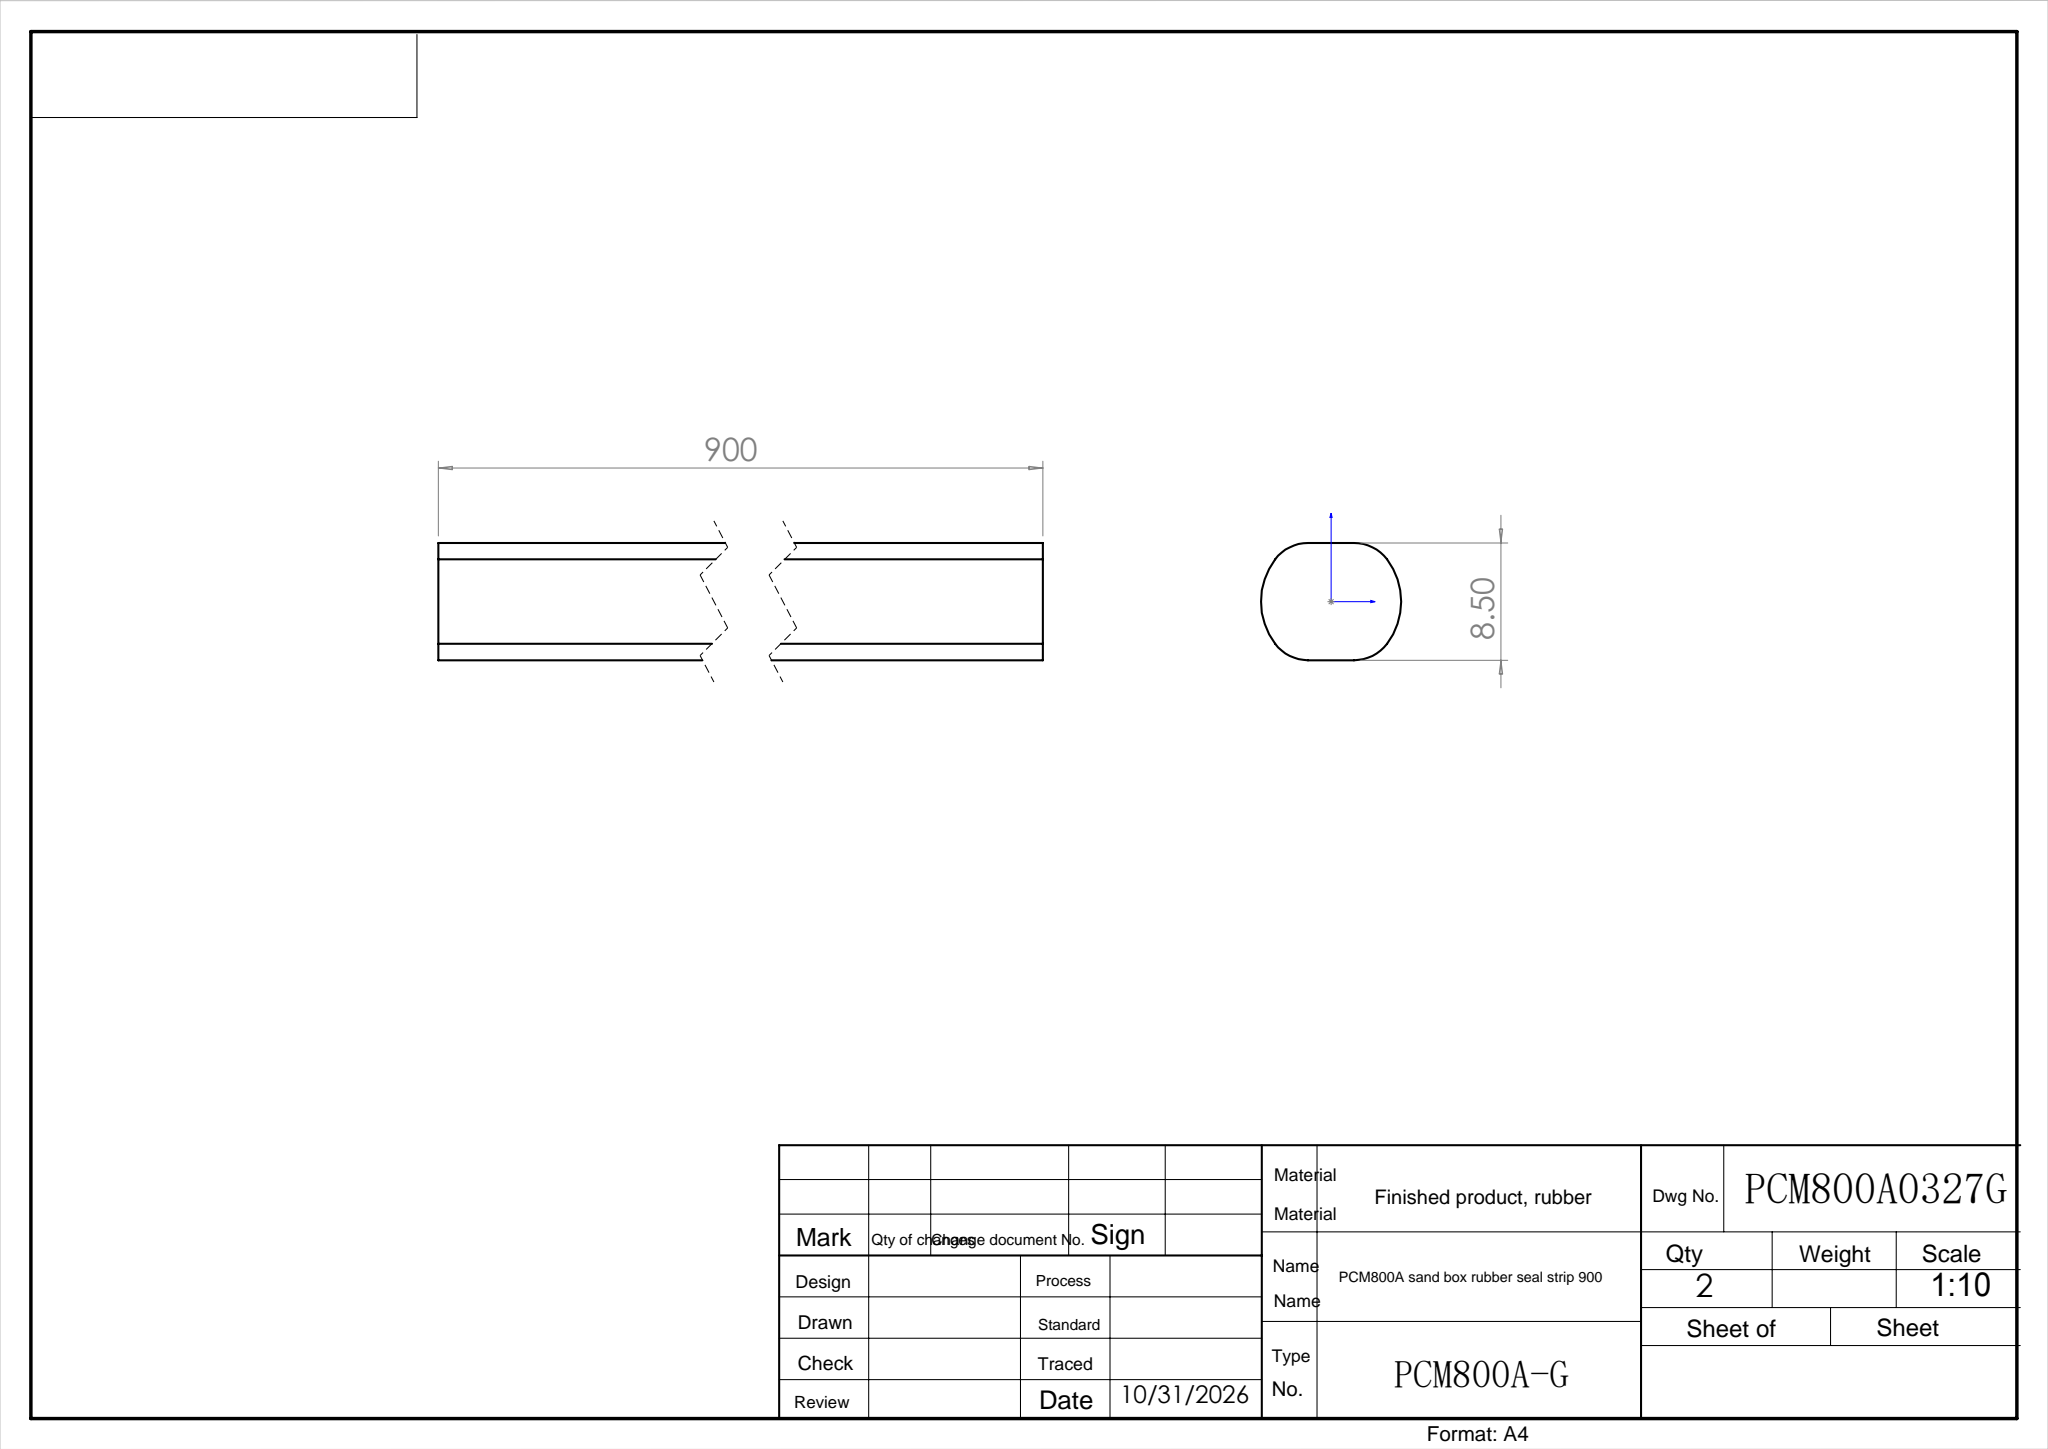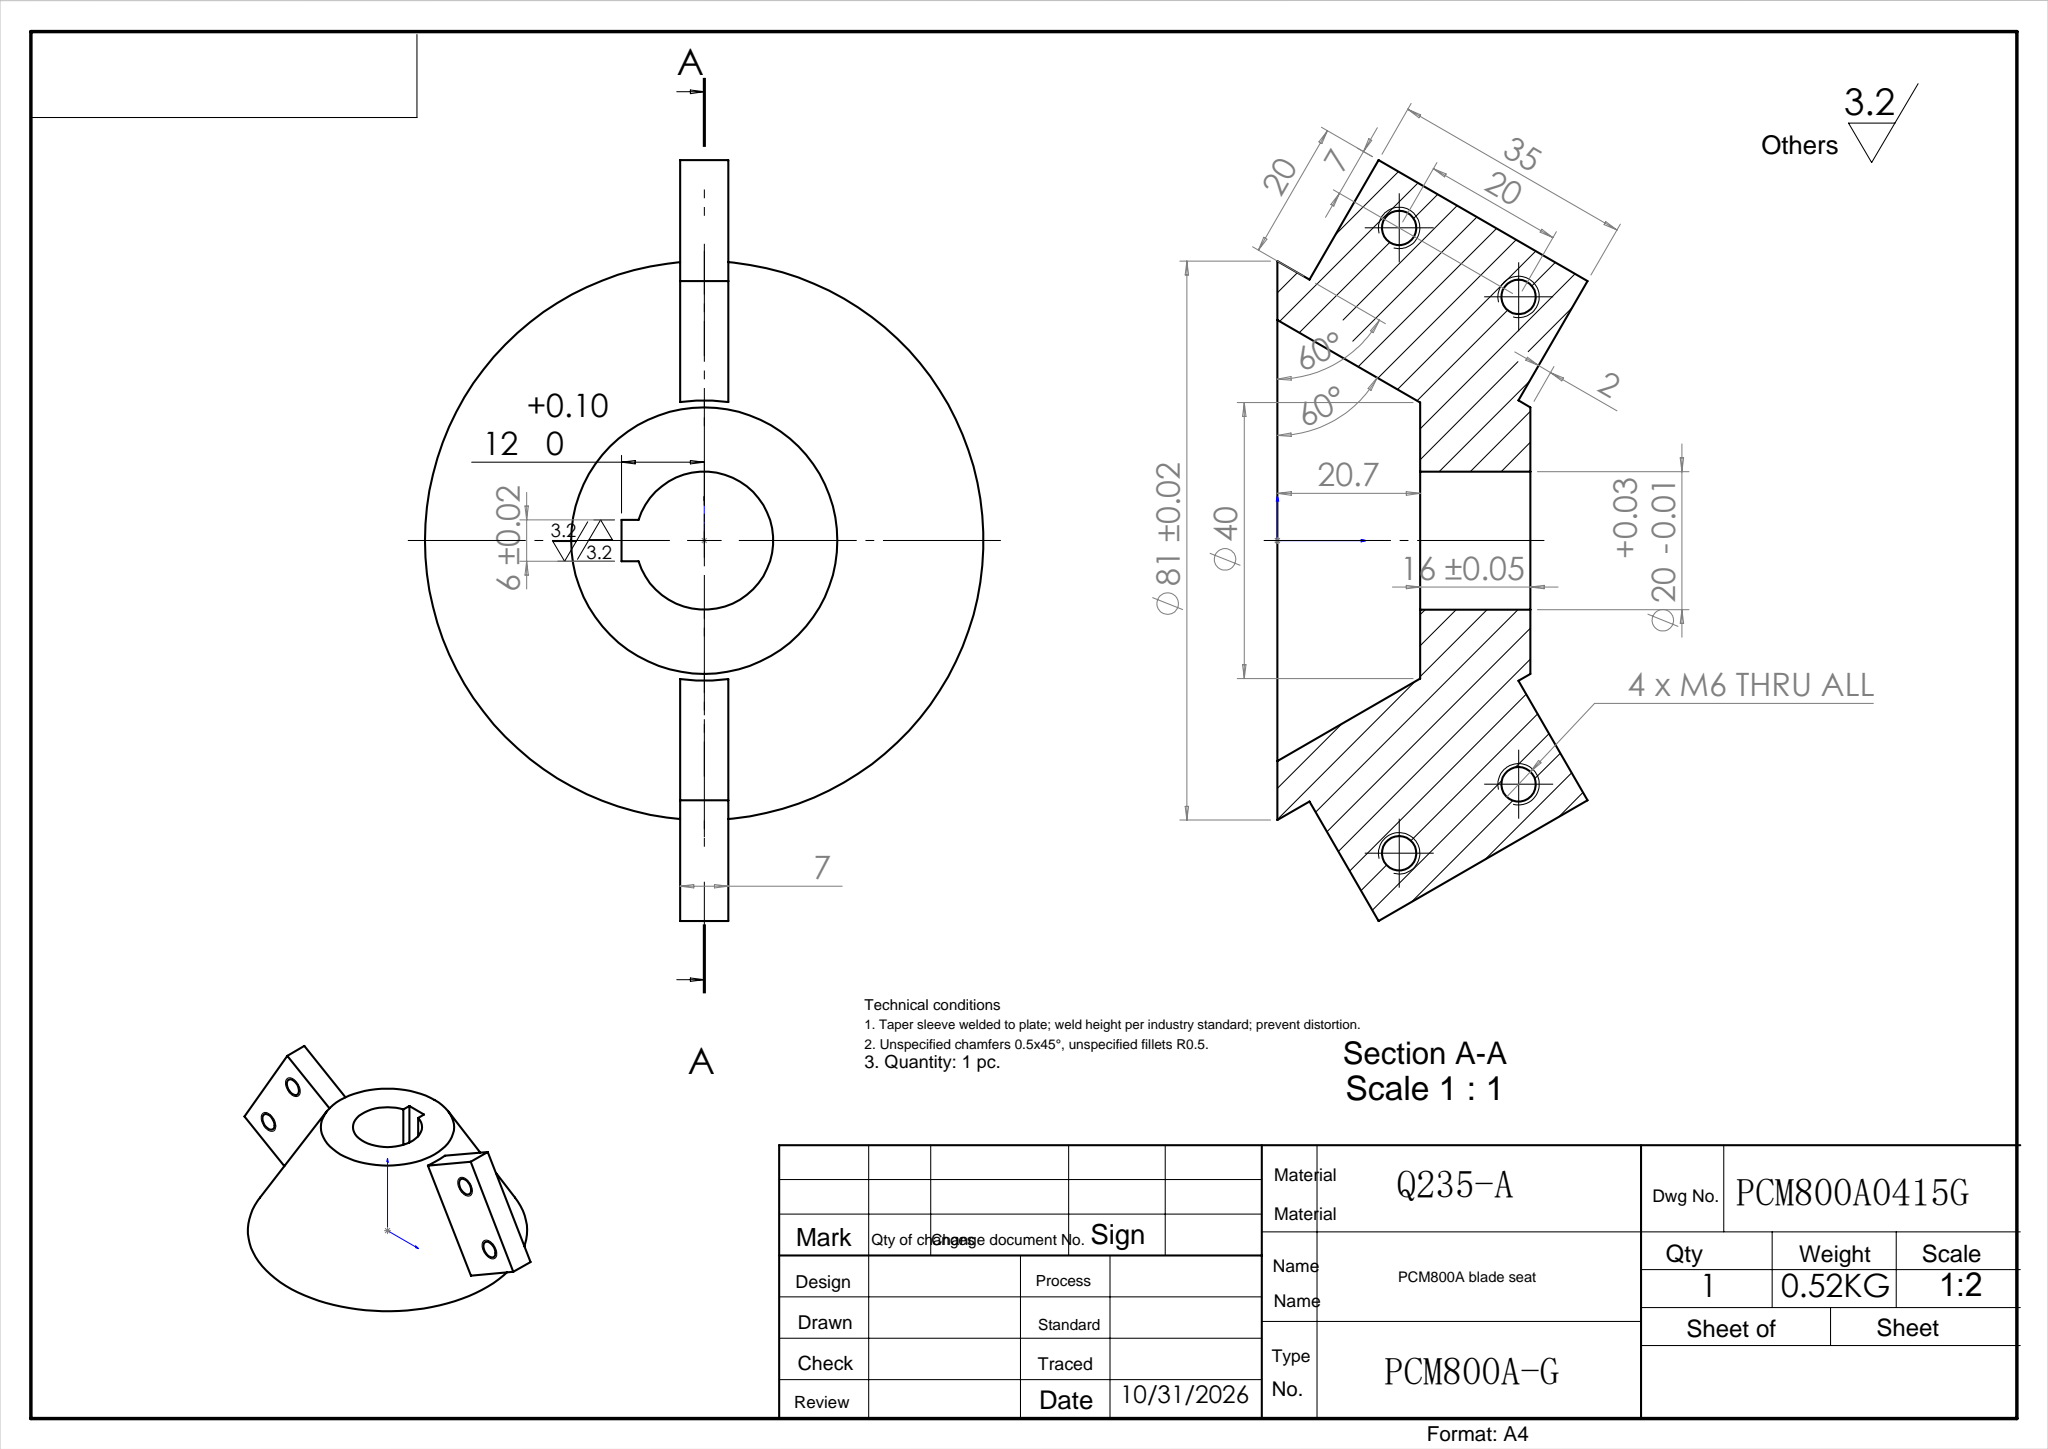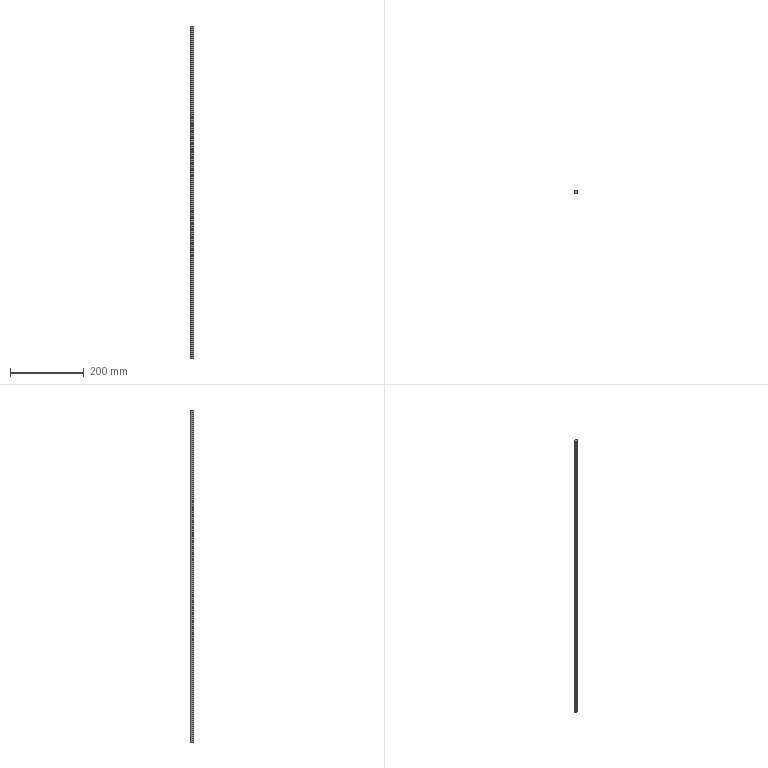Part | SolidWorks | features Extrusion 1 | 1 solid | 11 faces | box 10.158 x 8.5 x 900 mm | volume 66632 mm3 | cylinder 7 | plane 4 | commonest cylinder face diameters 6 x4 10.158 x3
STEP:
#1=CARTESIAN_POINT('',(-5.079,0.,900.));
#2=VERTEX_POINT('',#1);
#3=CARTESIAN_POINT('',(-4.059,-3.054,900.));
#4=VERTEX_POINT('',#3);
#5=CARTESIAN_POINT('',(0.,0.,900.));
#6=DIRECTION('',(0.,0.,1.));
#7=DIRECTION('',(1.,0.,0.));
#8=AXIS2_PLACEMENT_3D('',#5,#6,#7);
#9=CIRCLE('',#8,5.079);
#10=EDGE_CURVE('',#2,#4,#9,.T.);
#11=ORIENTED_EDGE('',*,*,#10,.F.);
#12=CARTESIAN_POINT('',(-5.079,0.,0.));
#13=VERTEX_POINT('',#12);
#14=CARTESIAN_POINT('',(-5.079,0.,900.));
#15=DIRECTION('',(0.,0.,-1.));
#16=VECTOR('',#15,1000.);
#17=LINE('',#14,#16);
#18=EDGE_CURVE('',#2,#13,#17,.T.);
#19=ORIENTED_EDGE('',*,*,#18,.T.);
#20=CARTESIAN_POINT('',(-4.059,-3.054,0.));
#21=VERTEX_POINT('',#20);
#22=CARTESIAN_POINT('',(0.,0.,0.));
#23=DIRECTION('',(0.,0.,1.));
#24=DIRECTION('',(1.,0.,0.));
#25=AXIS2_PLACEMENT_3D('',#22,#23,#24);
#26=CIRCLE('',#25,5.079);
#27=EDGE_CURVE('',#13,#21,#26,.T.);
#28=ORIENTED_EDGE('',*,*,#27,.T.);
#29=CARTESIAN_POINT('',(-4.059,-3.054,900.));
#30=DIRECTION('',(0.,0.,-1.));
#31=VECTOR('',#30,1000.);
#32=LINE('',#29,#31);
#33=EDGE_CURVE('',#4,#21,#32,.T.);
#34=ORIENTED_EDGE('',*,*,#33,.F.);
#35=EDGE_LOOP('',(#11,#19,#28,#34));
#36=FACE_OUTER_BOUND('',#35,.T.);
#37=CARTESIAN_POINT('',(0.,0.,900.));
#38=DIRECTION('',(0.,0.,-1.));
#39=DIRECTION('',(-1.,0.,0.));
#40=AXIS2_PLACEMENT_3D('',#37,#38,#39);
#41=CYLINDRICAL_SURFACE('',#40,5.079);
#42=ADVANCED_FACE('',(#36),#41,.T.);
#43=CARTESIAN_POINT('',(-1.661,4.25,0.));
#44=VERTEX_POINT('',#43);
#45=CARTESIAN_POINT('',(-4.059,3.054,0.));
#46=VERTEX_POINT('',#45);
#47=CARTESIAN_POINT('',(-1.661,1.25,0.));
#48=DIRECTION('',(0.,0.,1.));
#49=DIRECTION('',(-1.,0.,0.));
#50=AXIS2_PLACEMENT_3D('',#47,#48,#49);
#51=CIRCLE('',#50,3.);
#52=EDGE_CURVE('',#44,#46,#51,.T.);
#53=ORIENTED_EDGE('',*,*,#52,.T.);
#54=CARTESIAN_POINT('',(-4.059,3.054,900.));
#55=VERTEX_POINT('',#54);
#56=CARTESIAN_POINT('',(-4.059,3.054,900.));
#57=DIRECTION('',(0.,0.,-1.));
#58=VECTOR('',#57,1000.);
#59=LINE('',#56,#58);
#60=EDGE_CURVE('',#55,#46,#59,.T.);
#61=ORIENTED_EDGE('',*,*,#60,.F.);
#62=CARTESIAN_POINT('',(-1.661,4.25,900.));
#63=VERTEX_POINT('',#62);
#64=CARTESIAN_POINT('',(-1.661,1.25,900.));
#65=DIRECTION('',(0.,0.,1.));
#66=DIRECTION('',(-1.,0.,0.));
#67=AXIS2_PLACEMENT_3D('',#64,#65,#66);
#68=CIRCLE('',#67,3.);
#69=EDGE_CURVE('',#63,#55,#68,.T.);
#70=ORIENTED_EDGE('',*,*,#69,.F.);
#71=CARTESIAN_POINT('',(-1.661,4.25,900.));
#72=DIRECTION('',(0.,0.,-1.));
#73=VECTOR('',#72,1000.);
#74=LINE('',#71,#73);
#75=EDGE_CURVE('',#63,#44,#74,.T.);
#76=ORIENTED_EDGE('',*,*,#75,.T.);
#77=EDGE_LOOP('',(#53,#61,#70,#76));
#78=FACE_OUTER_BOUND('',#77,.T.);
#79=CARTESIAN_POINT('',(-1.661,1.25,900.));
#80=DIRECTION('',(0.,0.,-1.));
#81=DIRECTION('',(-1.,0.,0.));
#82=AXIS2_PLACEMENT_3D('',#79,#80,#81);
#83=CYLINDRICAL_SURFACE('',#82,3.);
#84=ADVANCED_FACE('',(#78),#83,.T.);
#85=ORIENTED_EDGE('',*,*,#18,.F.);
#86=CARTESIAN_POINT('',(0.,0.,900.));
#87=DIRECTION('',(0.,0.,1.));
#88=DIRECTION('',(1.,0.,0.));
#89=AXIS2_PLACEMENT_3D('',#86,#87,#88);
#90=CIRCLE('',#89,5.079);
#91=EDGE_CURVE('',#55,#2,#90,.T.);
#92=ORIENTED_EDGE('',*,*,#91,.F.);
#93=ORIENTED_EDGE('',*,*,#60,.T.);
#94=CARTESIAN_POINT('',(0.,0.,0.));
#95=DIRECTION('',(0.,0.,1.));
#96=DIRECTION('',(1.,0.,0.));
#97=AXIS2_PLACEMENT_3D('',#94,#95,#96);
#98=CIRCLE('',#97,5.079);
#99=EDGE_CURVE('',#46,#13,#98,.T.);
#100=ORIENTED_EDGE('',*,*,#99,.T.);
#101=EDGE_LOOP('',(#85,#92,#93,#100));
#102=FACE_OUTER_BOUND('',#101,.T.);
#103=CARTESIAN_POINT('',(0.,0.,900.));
#104=DIRECTION('',(0.,0.,-1.));
#105=DIRECTION('',(-1.,0.,0.));
#106=AXIS2_PLACEMENT_3D('',#103,#104,#105);
#107=CYLINDRICAL_SURFACE('',#106,5.079);
#108=ADVANCED_FACE('',(#102),#107,.T.);
#109=CARTESIAN_POINT('',(-1.661,-4.25,0.));
#110=VERTEX_POINT('',#109);
#111=CARTESIAN_POINT('',(-1.661,-1.25,0.));
#112=DIRECTION('',(0.,0.,1.));
#113=DIRECTION('',(1.,0.,0.));
#114=AXIS2_PLACEMENT_3D('',#111,#112,#113);
#115=CIRCLE('',#114,3.);
#116=EDGE_CURVE('',#21,#110,#115,.T.);
#117=ORIENTED_EDGE('',*,*,#116,.T.);
#118=CARTESIAN_POINT('',(-1.661,-4.25,900.));
#119=VERTEX_POINT('',#118);
#120=CARTESIAN_POINT('',(-1.661,-4.25,900.));
#121=DIRECTION('',(0.,0.,-1.));
#122=VECTOR('',#121,1000.);
#123=LINE('',#120,#122);
#124=EDGE_CURVE('',#119,#110,#123,.T.);
#125=ORIENTED_EDGE('',*,*,#124,.F.);
#126=CARTESIAN_POINT('',(-1.661,-1.25,900.));
#127=DIRECTION('',(0.,0.,1.));
#128=DIRECTION('',(1.,0.,0.));
#129=AXIS2_PLACEMENT_3D('',#126,#127,#128);
#130=CIRCLE('',#129,3.);
#131=EDGE_CURVE('',#4,#119,#130,.T.);
#132=ORIENTED_EDGE('',*,*,#131,.F.);
#133=ORIENTED_EDGE('',*,*,#33,.T.);
#134=EDGE_LOOP('',(#117,#125,#132,#133));
#135=FACE_OUTER_BOUND('',#134,.T.);
#136=CARTESIAN_POINT('',(-1.661,-1.25,900.));
#137=DIRECTION('',(0.,0.,-1.));
#138=DIRECTION('',(-1.,0.,0.));
#139=AXIS2_PLACEMENT_3D('',#136,#137,#138);
#140=CYLINDRICAL_SURFACE('',#139,3.);
#141=ADVANCED_FACE('',(#135),#140,.T.);
#142=CARTESIAN_POINT('',(1.661,-4.25,0.));
#143=VERTEX_POINT('',#142);
#144=CARTESIAN_POINT('',(-1.661,-4.25,0.));
#145=DIRECTION('',(1.,0.,0.));
#146=VECTOR('',#145,1000.);
#147=LINE('',#144,#146);
#148=EDGE_CURVE('',#110,#143,#147,.T.);
#149=ORIENTED_EDGE('',*,*,#148,.T.);
#150=CARTESIAN_POINT('',(1.661,-4.25,900.));
#151=VERTEX_POINT('',#150);
#152=CARTESIAN_POINT('',(1.661,-4.25,900.));
#153=DIRECTION('',(0.,0.,-1.));
#154=VECTOR('',#153,1000.);
#155=LINE('',#152,#154);
#156=EDGE_CURVE('',#151,#143,#155,.T.);
#157=ORIENTED_EDGE('',*,*,#156,.F.);
#158=CARTESIAN_POINT('',(-1.661,-4.25,900.));
#159=DIRECTION('',(1.,0.,0.));
#160=VECTOR('',#159,1000.);
#161=LINE('',#158,#160);
#162=EDGE_CURVE('',#119,#151,#161,.T.);
#163=ORIENTED_EDGE('',*,*,#162,.F.);
#164=ORIENTED_EDGE('',*,*,#124,.T.);
#165=EDGE_LOOP('',(#149,#157,#163,#164));
#166=FACE_OUTER_BOUND('',#165,.T.);
#167=CARTESIAN_POINT('',(-1.661,-4.25,900.));
#168=DIRECTION('',(0.,1.,0.));
#169=DIRECTION('',(0.,0.,1.));
#170=AXIS2_PLACEMENT_3D('',#167,#168,#169);
#171=PLANE('',#170);
#172=ADVANCED_FACE('',(#166),#171,.F.);
#173=CARTESIAN_POINT('',(4.059,-3.054,0.));
#174=VERTEX_POINT('',#173);
#175=CARTESIAN_POINT('',(1.661,-1.25,0.));
#176=DIRECTION('',(0.,0.,1.));
#177=DIRECTION('',(1.,0.,0.));
#178=AXIS2_PLACEMENT_3D('',#175,#176,#177);
#179=CIRCLE('',#178,3.);
#180=EDGE_CURVE('',#143,#174,#179,.T.);
#181=ORIENTED_EDGE('',*,*,#180,.T.);
#182=CARTESIAN_POINT('',(4.059,-3.054,900.));
#183=VERTEX_POINT('',#182);
#184=CARTESIAN_POINT('',(4.059,-3.054,900.));
#185=DIRECTION('',(0.,0.,-1.));
#186=VECTOR('',#185,1000.);
#187=LINE('',#184,#186);
#188=EDGE_CURVE('',#183,#174,#187,.T.);
#189=ORIENTED_EDGE('',*,*,#188,.F.);
#190=CARTESIAN_POINT('',(1.661,-1.25,900.));
#191=DIRECTION('',(0.,0.,1.));
#192=DIRECTION('',(1.,0.,0.));
#193=AXIS2_PLACEMENT_3D('',#190,#191,#192);
#194=CIRCLE('',#193,3.);
#195=EDGE_CURVE('',#151,#183,#194,.T.);
#196=ORIENTED_EDGE('',*,*,#195,.F.);
#197=ORIENTED_EDGE('',*,*,#156,.T.);
#198=EDGE_LOOP('',(#181,#189,#196,#197));
#199=FACE_OUTER_BOUND('',#198,.T.);
#200=CARTESIAN_POINT('',(1.661,-1.25,900.));
#201=DIRECTION('',(0.,0.,-1.));
#202=DIRECTION('',(-1.,0.,0.));
#203=AXIS2_PLACEMENT_3D('',#200,#201,#202);
#204=CYLINDRICAL_SURFACE('',#203,3.);
#205=ADVANCED_FACE('',(#199),#204,.T.);
#206=CARTESIAN_POINT('',(4.059,3.054,0.));
#207=VERTEX_POINT('',#206);
#208=CARTESIAN_POINT('',(0.,0.,0.));
#209=DIRECTION('',(0.,0.,1.));
#210=DIRECTION('',(1.,0.,0.));
#211=AXIS2_PLACEMENT_3D('',#208,#209,#210);
#212=CIRCLE('',#211,5.079);
#213=EDGE_CURVE('',#174,#207,#212,.T.);
#214=ORIENTED_EDGE('',*,*,#213,.T.);
#215=CARTESIAN_POINT('',(4.059,3.054,900.));
#216=VERTEX_POINT('',#215);
#217=CARTESIAN_POINT('',(4.059,3.054,900.));
#218=DIRECTION('',(0.,0.,-1.));
#219=VECTOR('',#218,1000.);
#220=LINE('',#217,#219);
#221=EDGE_CURVE('',#216,#207,#220,.T.);
#222=ORIENTED_EDGE('',*,*,#221,.F.);
#223=CARTESIAN_POINT('',(0.,0.,900.));
#224=DIRECTION('',(0.,0.,1.));
#225=DIRECTION('',(1.,0.,0.));
#226=AXIS2_PLACEMENT_3D('',#223,#224,#225);
#227=CIRCLE('',#226,5.079);
#228=EDGE_CURVE('',#183,#216,#227,.T.);
#229=ORIENTED_EDGE('',*,*,#228,.F.);
#230=ORIENTED_EDGE('',*,*,#188,.T.);
#231=EDGE_LOOP('',(#214,#222,#229,#230));
#232=FACE_OUTER_BOUND('',#231,.T.);
#233=CARTESIAN_POINT('',(0.,0.,900.));
#234=DIRECTION('',(0.,0.,-1.));
#235=DIRECTION('',(-1.,0.,0.));
#236=AXIS2_PLACEMENT_3D('',#233,#234,#235);
#237=CYLINDRICAL_SURFACE('',#236,5.079);
#238=ADVANCED_FACE('',(#232),#237,.T.);
#239=CARTESIAN_POINT('',(1.661,4.25,0.));
#240=VERTEX_POINT('',#239);
#241=CARTESIAN_POINT('',(1.661,1.25,0.));
#242=DIRECTION('',(0.,0.,1.));
#243=DIRECTION('',(1.,0.,0.));
#244=AXIS2_PLACEMENT_3D('',#241,#242,#243);
#245=CIRCLE('',#244,3.);
#246=EDGE_CURVE('',#207,#240,#245,.T.);
#247=ORIENTED_EDGE('',*,*,#246,.T.);
#248=CARTESIAN_POINT('',(1.661,4.25,900.));
#249=VERTEX_POINT('',#248);
#250=CARTESIAN_POINT('',(1.661,4.25,900.));
#251=DIRECTION('',(0.,0.,-1.));
#252=VECTOR('',#251,1000.);
#253=LINE('',#250,#252);
#254=EDGE_CURVE('',#249,#240,#253,.T.);
#255=ORIENTED_EDGE('',*,*,#254,.F.);
#256=CARTESIAN_POINT('',(1.661,1.25,900.));
#257=DIRECTION('',(0.,0.,1.));
#258=DIRECTION('',(1.,0.,0.));
#259=AXIS2_PLACEMENT_3D('',#256,#257,#258);
#260=CIRCLE('',#259,3.);
#261=EDGE_CURVE('',#216,#249,#260,.T.);
#262=ORIENTED_EDGE('',*,*,#261,.F.);
#263=ORIENTED_EDGE('',*,*,#221,.T.);
#264=EDGE_LOOP('',(#247,#255,#262,#263));
#265=FACE_OUTER_BOUND('',#264,.T.);
#266=CARTESIAN_POINT('',(1.661,1.25,900.));
#267=DIRECTION('',(0.,0.,-1.));
#268=DIRECTION('',(-1.,0.,0.));
#269=AXIS2_PLACEMENT_3D('',#266,#267,#268);
#270=CYLINDRICAL_SURFACE('',#269,3.);
#271=ADVANCED_FACE('',(#265),#270,.T.);
#272=CARTESIAN_POINT('',(-1.661,4.25,0.));
#273=DIRECTION('',(-1.,0.,0.));
#274=VECTOR('',#273,1000.);
#275=LINE('',#272,#274);
#276=EDGE_CURVE('',#240,#44,#275,.T.);
#277=ORIENTED_EDGE('',*,*,#276,.T.);
#278=ORIENTED_EDGE('',*,*,#75,.F.);
#279=CARTESIAN_POINT('',(-1.661,4.25,900.));
#280=DIRECTION('',(-1.,0.,0.));
#281=VECTOR('',#280,1000.);
#282=LINE('',#279,#281);
#283=EDGE_CURVE('',#249,#63,#282,.T.);
#284=ORIENTED_EDGE('',*,*,#283,.F.);
#285=ORIENTED_EDGE('',*,*,#254,.T.);
#286=EDGE_LOOP('',(#277,#278,#284,#285));
#287=FACE_OUTER_BOUND('',#286,.T.);
#288=CARTESIAN_POINT('',(-1.661,4.25,900.));
#289=DIRECTION('',(0.,-1.,0.));
#290=DIRECTION('',(0.,0.,-1.));
#291=AXIS2_PLACEMENT_3D('',#288,#289,#290);
#292=PLANE('',#291);
#293=ADVANCED_FACE('',(#287),#292,.F.);
#294=ORIENTED_EDGE('',*,*,#69,.T.);
#295=ORIENTED_EDGE('',*,*,#91,.T.);
#296=ORIENTED_EDGE('',*,*,#10,.T.);
#297=ORIENTED_EDGE('',*,*,#131,.T.);
#298=ORIENTED_EDGE('',*,*,#162,.T.);
#299=ORIENTED_EDGE('',*,*,#195,.T.);
#300=ORIENTED_EDGE('',*,*,#228,.T.);
#301=ORIENTED_EDGE('',*,*,#261,.T.);
#302=ORIENTED_EDGE('',*,*,#283,.T.);
#303=EDGE_LOOP('',(#294,#295,#296,#297,#298,#299,#300,#301,#302));
#304=FACE_OUTER_BOUND('',#303,.T.);
#305=CARTESIAN_POINT('',(-1.661,1.25,900.));
#306=DIRECTION('',(0.,0.,-1.));
#307=DIRECTION('',(-1.,0.,0.));
#308=AXIS2_PLACEMENT_3D('',#305,#306,#307);
#309=PLANE('',#308);
#310=ADVANCED_FACE('',(#304),#309,.F.);
#311=ORIENTED_EDGE('',*,*,#52,.F.);
#312=ORIENTED_EDGE('',*,*,#276,.F.);
#313=ORIENTED_EDGE('',*,*,#246,.F.);
#314=ORIENTED_EDGE('',*,*,#213,.F.);
#315=ORIENTED_EDGE('',*,*,#180,.F.);
#316=ORIENTED_EDGE('',*,*,#148,.F.);
#317=ORIENTED_EDGE('',*,*,#116,.F.);
#318=ORIENTED_EDGE('',*,*,#27,.F.);
#319=ORIENTED_EDGE('',*,*,#99,.F.);
#320=EDGE_LOOP('',(#311,#312,#313,#314,#315,#316,#317,#318,#319));
#321=FACE_OUTER_BOUND('',#320,.T.);
#322=CARTESIAN_POINT('',(-1.661,1.25,0.));
#323=DIRECTION('',(0.,0.,-1.));
#324=DIRECTION('',(-1.,0.,0.));
#325=AXIS2_PLACEMENT_3D('',#322,#323,#324);
#326=PLANE('',#325);
#327=ADVANCED_FACE('',(#321),#326,.T.);
#328=CLOSED_SHELL('',(#42,#84,#108,#141,#172,#205,#238,#271,#293,#310,#327));
#329=MANIFOLD_SOLID_BREP('',#328);
#330=CARTESIAN_POINT('',(0.,0.,0.));
#331=DIRECTION('',(0.,0.,1.));
#332=DIRECTION('',(1.,0.,0.));
#333=AXIS2_PLACEMENT_3D('',#330,#331,#332);
#334=(LENGTH_UNIT()NAMED_UNIT(*)SI_UNIT(.MILLI.,.METRE.));
#335=UNCERTAINTY_MEASURE_WITH_UNIT(LENGTH_MEASURE(0.00001),#334,'','');
#336=(NAMED_UNIT(*)PLANE_ANGLE_UNIT()SI_UNIT($,.RADIAN.));
#337=(NAMED_UNIT(*)SI_UNIT($,.STERADIAN.)SOLID_ANGLE_UNIT());
#338=(GEOMETRIC_REPRESENTATION_CONTEXT(3)GLOBAL_UNCERTAINTY_ASSIGNED_CONTEXT((#335))GLOBAL_UNIT_ASSIGNED_CONTEXT((#334,#336,#337))REPRESENTATION_CONTEXT('',''));
#339=ADVANCED_BREP_SHAPE_REPRESENTATION('',(#329,#333),#338);